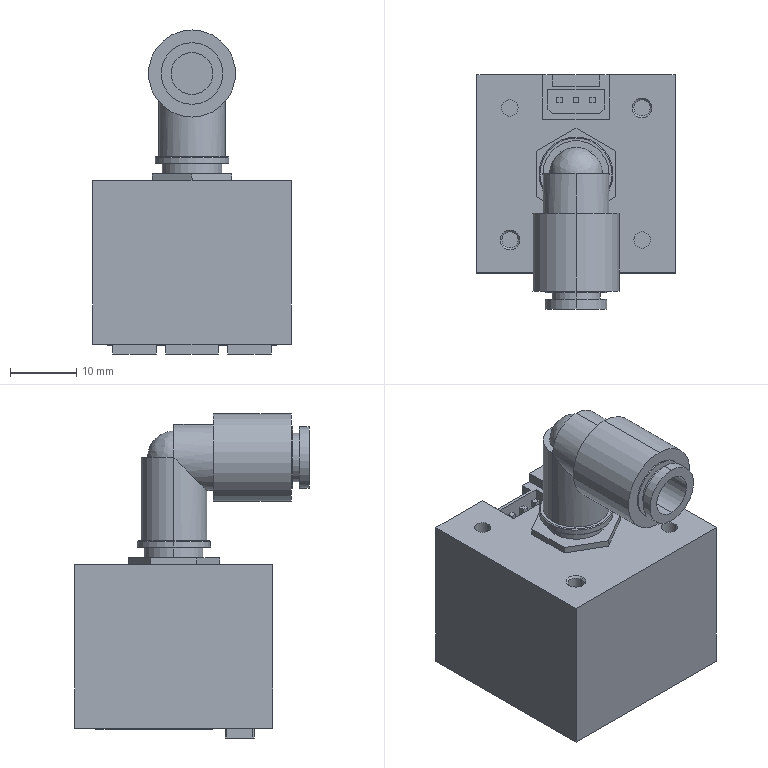Part | SolidWorks | features BaseBody 1 | 1 solid | 112 faces | box 30 x 35.5 x 49.1 mm | volume 25063 mm3 | plane 77 | cylinder 26 | cone 8 | spline 1 | commonest cylinder face diameters 2.46 x4 2.5 x4 9.35 x4 10 x4 6.35 x2 7.35 x2